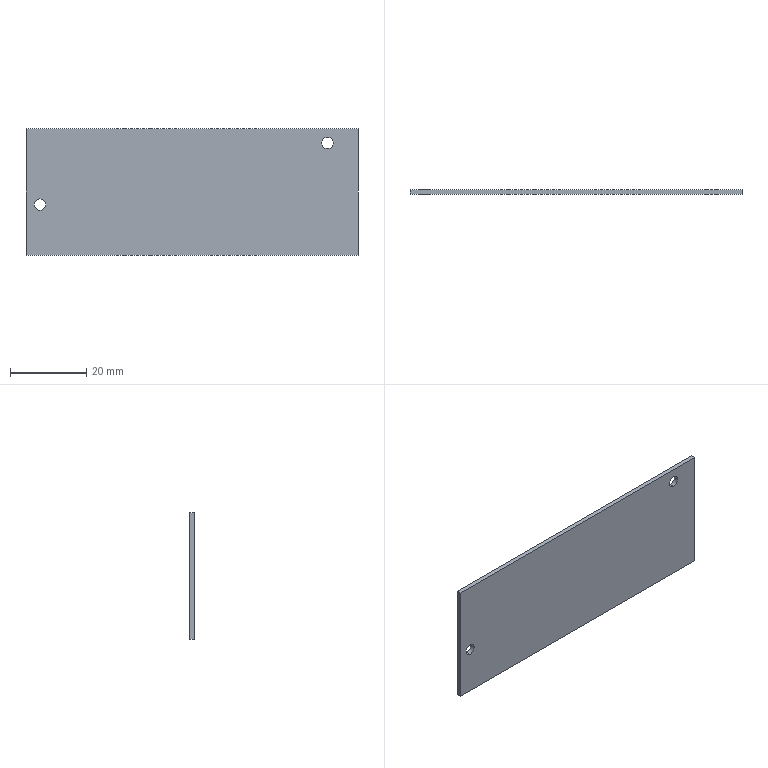Part | SolidWorks | features BaseBody 1 | 1 solid | 10 faces | box 87 x 1.2 x 33.1 mm | volume 3439 mm3 | plane 6 | cylinder 4 | commonest cylinder face diameters 3 x4
STEP:
#1=CARTESIAN_POINT('',(35.52,0.,14.34));
#2=VERTEX_POINT('',#1);
#3=CARTESIAN_POINT('',(35.52,0.,11.34));
#4=VERTEX_POINT('',#3);
#5=CARTESIAN_POINT('',(35.52,0.,12.84));
#6=DIRECTION('',(0.,-1.,0.));
#7=DIRECTION('',(0.,0.,1.));
#8=AXIS2_PLACEMENT_3D('',#5,#6,#7);
#9=CIRCLE('',#8,1.5);
#10=EDGE_CURVE('',#2,#4,#9,.T.);
#11=ORIENTED_EDGE('',*,*,#10,.T.);
#12=CARTESIAN_POINT('',(35.52,1.2,11.34));
#13=VERTEX_POINT('',#12);
#14=CARTESIAN_POINT('',(35.52,0.,11.34));
#15=DIRECTION('',(0.,1.,0.));
#16=VECTOR('',#15,1000.);
#17=LINE('',#14,#16);
#18=EDGE_CURVE('',#4,#13,#17,.T.);
#19=ORIENTED_EDGE('',*,*,#18,.T.);
#20=CARTESIAN_POINT('',(35.52,1.2,14.34));
#21=VERTEX_POINT('',#20);
#22=CARTESIAN_POINT('',(35.52,1.2,12.84));
#23=DIRECTION('',(0.,-1.,0.));
#24=DIRECTION('',(0.,0.,1.));
#25=AXIS2_PLACEMENT_3D('',#22,#23,#24);
#26=CIRCLE('',#25,1.5);
#27=EDGE_CURVE('',#21,#13,#26,.T.);
#28=ORIENTED_EDGE('',*,*,#27,.F.);
#29=CARTESIAN_POINT('',(35.52,0.,14.34));
#30=DIRECTION('',(0.,1.,0.));
#31=VECTOR('',#30,1000.);
#32=LINE('',#29,#31);
#33=EDGE_CURVE('',#2,#21,#32,.T.);
#34=ORIENTED_EDGE('',*,*,#33,.F.);
#35=EDGE_LOOP('',(#11,#19,#28,#34));
#36=FACE_OUTER_BOUND('',#35,.T.);
#37=CARTESIAN_POINT('',(35.52,0.,12.84));
#38=DIRECTION('',(0.,1.,0.));
#39=DIRECTION('',(0.,0.,1.));
#40=AXIS2_PLACEMENT_3D('',#37,#38,#39);
#41=CYLINDRICAL_SURFACE('',#40,1.5);
#42=ADVANCED_FACE('',(#36),#41,.F.);
#43=CARTESIAN_POINT('',(-39.87,0.,-1.82));
#44=VERTEX_POINT('',#43);
#45=CARTESIAN_POINT('',(-39.87,0.,-4.82));
#46=VERTEX_POINT('',#45);
#47=CARTESIAN_POINT('',(-39.87,0.,-3.32));
#48=DIRECTION('',(0.,-1.,0.));
#49=DIRECTION('',(0.,0.,1.));
#50=AXIS2_PLACEMENT_3D('',#47,#48,#49);
#51=CIRCLE('',#50,1.5);
#52=EDGE_CURVE('',#44,#46,#51,.T.);
#53=ORIENTED_EDGE('',*,*,#52,.T.);
#54=CARTESIAN_POINT('',(-39.87,1.2,-4.82));
#55=VERTEX_POINT('',#54);
#56=CARTESIAN_POINT('',(-39.87,0.,-4.82));
#57=DIRECTION('',(0.,1.,0.));
#58=VECTOR('',#57,1000.);
#59=LINE('',#56,#58);
#60=EDGE_CURVE('',#46,#55,#59,.T.);
#61=ORIENTED_EDGE('',*,*,#60,.T.);
#62=CARTESIAN_POINT('',(-39.87,1.2,-1.82));
#63=VERTEX_POINT('',#62);
#64=CARTESIAN_POINT('',(-39.87,1.2,-3.32));
#65=DIRECTION('',(0.,-1.,0.));
#66=DIRECTION('',(0.,0.,1.));
#67=AXIS2_PLACEMENT_3D('',#64,#65,#66);
#68=CIRCLE('',#67,1.5);
#69=EDGE_CURVE('',#63,#55,#68,.T.);
#70=ORIENTED_EDGE('',*,*,#69,.F.);
#71=CARTESIAN_POINT('',(-39.87,0.,-1.82));
#72=DIRECTION('',(0.,1.,0.));
#73=VECTOR('',#72,1000.);
#74=LINE('',#71,#73);
#75=EDGE_CURVE('',#44,#63,#74,.T.);
#76=ORIENTED_EDGE('',*,*,#75,.F.);
#77=EDGE_LOOP('',(#53,#61,#70,#76));
#78=FACE_OUTER_BOUND('',#77,.T.);
#79=CARTESIAN_POINT('',(-39.87,0.,-3.32));
#80=DIRECTION('',(0.,1.,0.));
#81=DIRECTION('',(0.,0.,1.));
#82=AXIS2_PLACEMENT_3D('',#79,#80,#81);
#83=CYLINDRICAL_SURFACE('',#82,1.5);
#84=ADVANCED_FACE('',(#78),#83,.F.);
#85=ORIENTED_EDGE('',*,*,#10,.F.);
#86=CARTESIAN_POINT('',(35.52,0.,12.84));
#87=DIRECTION('',(0.,-1.,0.));
#88=DIRECTION('',(0.,0.,1.));
#89=AXIS2_PLACEMENT_3D('',#86,#87,#88);
#90=CIRCLE('',#89,1.5);
#91=EDGE_CURVE('',#4,#2,#90,.T.);
#92=ORIENTED_EDGE('',*,*,#91,.F.);
#93=EDGE_LOOP('',(#85,#92));
#94=FACE_BOUND('',#93,.T.);
#95=ORIENTED_EDGE('',*,*,#52,.F.);
#96=CARTESIAN_POINT('',(-39.87,0.,-3.32));
#97=DIRECTION('',(0.,-1.,0.));
#98=DIRECTION('',(0.,0.,1.));
#99=AXIS2_PLACEMENT_3D('',#96,#97,#98);
#100=CIRCLE('',#99,1.5);
#101=EDGE_CURVE('',#46,#44,#100,.T.);
#102=ORIENTED_EDGE('',*,*,#101,.F.);
#103=EDGE_LOOP('',(#95,#102));
#104=FACE_BOUND('',#103,.T.);
#105=CARTESIAN_POINT('',(43.5,0.,16.55));
#106=VERTEX_POINT('',#105);
#107=CARTESIAN_POINT('',(43.5,0.,-16.55));
#108=VERTEX_POINT('',#107);
#109=CARTESIAN_POINT('',(43.5,0.,0.));
#110=DIRECTION('',(0.,0.,-1.));
#111=VECTOR('',#110,1000.);
#112=LINE('',#109,#111);
#113=EDGE_CURVE('',#106,#108,#112,.T.);
#114=ORIENTED_EDGE('',*,*,#113,.F.);
#115=CARTESIAN_POINT('',(-43.5,0.,16.55));
#116=VERTEX_POINT('',#115);
#117=CARTESIAN_POINT('',(0.,0.,16.55));
#118=DIRECTION('',(1.,0.,0.));
#119=VECTOR('',#118,1000.);
#120=LINE('',#117,#119);
#121=EDGE_CURVE('',#116,#106,#120,.T.);
#122=ORIENTED_EDGE('',*,*,#121,.F.);
#123=CARTESIAN_POINT('',(-43.5,0.,-16.55));
#124=VERTEX_POINT('',#123);
#125=CARTESIAN_POINT('',(-43.5,0.,0.));
#126=DIRECTION('',(0.,0.,1.));
#127=VECTOR('',#126,1000.);
#128=LINE('',#125,#127);
#129=EDGE_CURVE('',#124,#116,#128,.T.);
#130=ORIENTED_EDGE('',*,*,#129,.F.);
#131=CARTESIAN_POINT('',(0.,0.,-16.55));
#132=DIRECTION('',(-1.,0.,0.));
#133=VECTOR('',#132,1000.);
#134=LINE('',#131,#133);
#135=EDGE_CURVE('',#108,#124,#134,.T.);
#136=ORIENTED_EDGE('',*,*,#135,.F.);
#137=EDGE_LOOP('',(#114,#122,#130,#136));
#138=FACE_OUTER_BOUND('',#137,.T.);
#139=CARTESIAN_POINT('',(0.,0.,0.));
#140=DIRECTION('',(0.,1.,0.));
#141=DIRECTION('',(0.,0.,1.));
#142=AXIS2_PLACEMENT_3D('',#139,#140,#141);
#143=PLANE('',#142);
#144=ADVANCED_FACE('',(#94,#104,#138),#143,.F.);
#145=ORIENTED_EDGE('',*,*,#18,.F.);
#146=ORIENTED_EDGE('',*,*,#91,.T.);
#147=ORIENTED_EDGE('',*,*,#33,.T.);
#148=CARTESIAN_POINT('',(35.52,1.2,12.84));
#149=DIRECTION('',(0.,-1.,0.));
#150=DIRECTION('',(0.,0.,1.));
#151=AXIS2_PLACEMENT_3D('',#148,#149,#150);
#152=CIRCLE('',#151,1.5);
#153=EDGE_CURVE('',#13,#21,#152,.T.);
#154=ORIENTED_EDGE('',*,*,#153,.F.);
#155=EDGE_LOOP('',(#145,#146,#147,#154));
#156=FACE_OUTER_BOUND('',#155,.T.);
#157=CARTESIAN_POINT('',(35.52,0.,12.84));
#158=DIRECTION('',(0.,1.,0.));
#159=DIRECTION('',(0.,0.,1.));
#160=AXIS2_PLACEMENT_3D('',#157,#158,#159);
#161=CYLINDRICAL_SURFACE('',#160,1.5);
#162=ADVANCED_FACE('',(#156),#161,.F.);
#163=ORIENTED_EDGE('',*,*,#60,.F.);
#164=ORIENTED_EDGE('',*,*,#101,.T.);
#165=ORIENTED_EDGE('',*,*,#75,.T.);
#166=CARTESIAN_POINT('',(-39.87,1.2,-3.32));
#167=DIRECTION('',(0.,-1.,0.));
#168=DIRECTION('',(0.,0.,1.));
#169=AXIS2_PLACEMENT_3D('',#166,#167,#168);
#170=CIRCLE('',#169,1.5);
#171=EDGE_CURVE('',#55,#63,#170,.T.);
#172=ORIENTED_EDGE('',*,*,#171,.F.);
#173=EDGE_LOOP('',(#163,#164,#165,#172));
#174=FACE_OUTER_BOUND('',#173,.T.);
#175=CARTESIAN_POINT('',(-39.87,0.,-3.32));
#176=DIRECTION('',(0.,1.,0.));
#177=DIRECTION('',(0.,0.,1.));
#178=AXIS2_PLACEMENT_3D('',#175,#176,#177);
#179=CYLINDRICAL_SURFACE('',#178,1.5);
#180=ADVANCED_FACE('',(#174),#179,.F.);
#181=CARTESIAN_POINT('',(43.5,1.2,-16.55));
#182=VERTEX_POINT('',#181);
#183=CARTESIAN_POINT('',(43.5,0.,-16.55));
#184=DIRECTION('',(0.,-1.,0.));
#185=VECTOR('',#184,1000.);
#186=LINE('',#183,#185);
#187=EDGE_CURVE('',#182,#108,#186,.T.);
#188=ORIENTED_EDGE('',*,*,#187,.T.);
#189=ORIENTED_EDGE('',*,*,#135,.T.);
#190=CARTESIAN_POINT('',(-43.5,1.2,-16.55));
#191=VERTEX_POINT('',#190);
#192=CARTESIAN_POINT('',(-43.5,0.,-16.55));
#193=DIRECTION('',(0.,1.,0.));
#194=VECTOR('',#193,1000.);
#195=LINE('',#192,#194);
#196=EDGE_CURVE('',#124,#191,#195,.T.);
#197=ORIENTED_EDGE('',*,*,#196,.T.);
#198=CARTESIAN_POINT('',(43.5,1.2,-16.55));
#199=DIRECTION('',(1.,0.,0.));
#200=VECTOR('',#199,1000.);
#201=LINE('',#198,#200);
#202=EDGE_CURVE('',#191,#182,#201,.T.);
#203=ORIENTED_EDGE('',*,*,#202,.T.);
#204=EDGE_LOOP('',(#188,#189,#197,#203));
#205=FACE_OUTER_BOUND('',#204,.T.);
#206=CARTESIAN_POINT('',(43.5,0.,-16.55));
#207=DIRECTION('',(0.,0.,-1.));
#208=DIRECTION('',(-1.,0.,0.));
#209=AXIS2_PLACEMENT_3D('',#206,#207,#208);
#210=PLANE('',#209);
#211=ADVANCED_FACE('',(#205),#210,.T.);
#212=CARTESIAN_POINT('',(43.5,1.2,16.55));
#213=VERTEX_POINT('',#212);
#214=CARTESIAN_POINT('',(43.5,0.,16.55));
#215=DIRECTION('',(0.,-1.,0.));
#216=VECTOR('',#215,1000.);
#217=LINE('',#214,#216);
#218=EDGE_CURVE('',#213,#106,#217,.T.);
#219=ORIENTED_EDGE('',*,*,#218,.T.);
#220=ORIENTED_EDGE('',*,*,#113,.T.);
#221=ORIENTED_EDGE('',*,*,#187,.F.);
#222=CARTESIAN_POINT('',(43.5,1.2,16.55));
#223=DIRECTION('',(0.,0.,1.));
#224=VECTOR('',#223,1000.);
#225=LINE('',#222,#224);
#226=EDGE_CURVE('',#182,#213,#225,.T.);
#227=ORIENTED_EDGE('',*,*,#226,.T.);
#228=EDGE_LOOP('',(#219,#220,#221,#227));
#229=FACE_OUTER_BOUND('',#228,.T.);
#230=CARTESIAN_POINT('',(43.5,0.,16.55));
#231=DIRECTION('',(1.,0.,0.));
#232=DIRECTION('',(0.,0.,-1.));
#233=AXIS2_PLACEMENT_3D('',#230,#231,#232);
#234=PLANE('',#233);
#235=ADVANCED_FACE('',(#229),#234,.T.);
#236=CARTESIAN_POINT('',(-43.5,1.2,16.55));
#237=VERTEX_POINT('',#236);
#238=CARTESIAN_POINT('',(-43.5,0.,16.55));
#239=DIRECTION('',(0.,-1.,0.));
#240=VECTOR('',#239,1000.);
#241=LINE('',#238,#240);
#242=EDGE_CURVE('',#237,#116,#241,.T.);
#243=ORIENTED_EDGE('',*,*,#242,.T.);
#244=ORIENTED_EDGE('',*,*,#121,.T.);
#245=ORIENTED_EDGE('',*,*,#218,.F.);
#246=CARTESIAN_POINT('',(-43.5,1.2,16.55));
#247=DIRECTION('',(-1.,0.,0.));
#248=VECTOR('',#247,1000.);
#249=LINE('',#246,#248);
#250=EDGE_CURVE('',#213,#237,#249,.T.);
#251=ORIENTED_EDGE('',*,*,#250,.T.);
#252=EDGE_LOOP('',(#243,#244,#245,#251));
#253=FACE_OUTER_BOUND('',#252,.T.);
#254=CARTESIAN_POINT('',(-43.5,0.,16.55));
#255=DIRECTION('',(0.,0.,1.));
#256=DIRECTION('',(1.,0.,0.));
#257=AXIS2_PLACEMENT_3D('',#254,#255,#256);
#258=PLANE('',#257);
#259=ADVANCED_FACE('',(#253),#258,.T.);
#260=ORIENTED_EDGE('',*,*,#196,.F.);
#261=ORIENTED_EDGE('',*,*,#129,.T.);
#262=ORIENTED_EDGE('',*,*,#242,.F.);
#263=CARTESIAN_POINT('',(-43.5,1.2,-16.55));
#264=DIRECTION('',(0.,0.,-1.));
#265=VECTOR('',#264,1000.);
#266=LINE('',#263,#265);
#267=EDGE_CURVE('',#237,#191,#266,.T.);
#268=ORIENTED_EDGE('',*,*,#267,.T.);
#269=EDGE_LOOP('',(#260,#261,#262,#268));
#270=FACE_OUTER_BOUND('',#269,.T.);
#271=CARTESIAN_POINT('',(-43.5,0.,-16.55));
#272=DIRECTION('',(-1.,0.,0.));
#273=DIRECTION('',(0.,0.,1.));
#274=AXIS2_PLACEMENT_3D('',#271,#272,#273);
#275=PLANE('',#274);
#276=ADVANCED_FACE('',(#270),#275,.T.);
#277=ORIENTED_EDGE('',*,*,#27,.T.);
#278=ORIENTED_EDGE('',*,*,#153,.T.);
#279=EDGE_LOOP('',(#277,#278));
#280=FACE_BOUND('',#279,.T.);
#281=ORIENTED_EDGE('',*,*,#69,.T.);
#282=ORIENTED_EDGE('',*,*,#171,.T.);
#283=EDGE_LOOP('',(#281,#282));
#284=FACE_BOUND('',#283,.T.);
#285=ORIENTED_EDGE('',*,*,#202,.F.);
#286=ORIENTED_EDGE('',*,*,#267,.F.);
#287=ORIENTED_EDGE('',*,*,#250,.F.);
#288=ORIENTED_EDGE('',*,*,#226,.F.);
#289=EDGE_LOOP('',(#285,#286,#287,#288));
#290=FACE_OUTER_BOUND('',#289,.T.);
#291=CARTESIAN_POINT('',(0.,1.2,0.));
#292=DIRECTION('',(0.,1.,0.));
#293=DIRECTION('',(0.,0.,1.));
#294=AXIS2_PLACEMENT_3D('',#291,#292,#293);
#295=PLANE('',#294);
#296=ADVANCED_FACE('',(#280,#284,#290),#295,.T.);
#297=CLOSED_SHELL('',(#42,#84,#144,#162,#180,#211,#235,#259,#276,#296));
#298=MANIFOLD_SOLID_BREP('',#297);
#299=CARTESIAN_POINT('',(0.,0.,0.));
#300=DIRECTION('',(0.,0.,1.));
#301=DIRECTION('',(1.,0.,0.));
#302=AXIS2_PLACEMENT_3D('',#299,#300,#301);
#303=(LENGTH_UNIT()NAMED_UNIT(*)SI_UNIT(.MILLI.,.METRE.));
#304=UNCERTAINTY_MEASURE_WITH_UNIT(LENGTH_MEASURE(0.00001),#303,'','');
#305=(NAMED_UNIT(*)PLANE_ANGLE_UNIT()SI_UNIT($,.RADIAN.));
#306=(NAMED_UNIT(*)SI_UNIT($,.STERADIAN.)SOLID_ANGLE_UNIT());
#307=(GEOMETRIC_REPRESENTATION_CONTEXT(3)GLOBAL_UNCERTAINTY_ASSIGNED_CONTEXT((#304))GLOBAL_UNIT_ASSIGNED_CONTEXT((#303,#305,#306))REPRESENTATION_CONTEXT('',''));
#308=ADVANCED_BREP_SHAPE_REPRESENTATION('',(#298,#302),#307);